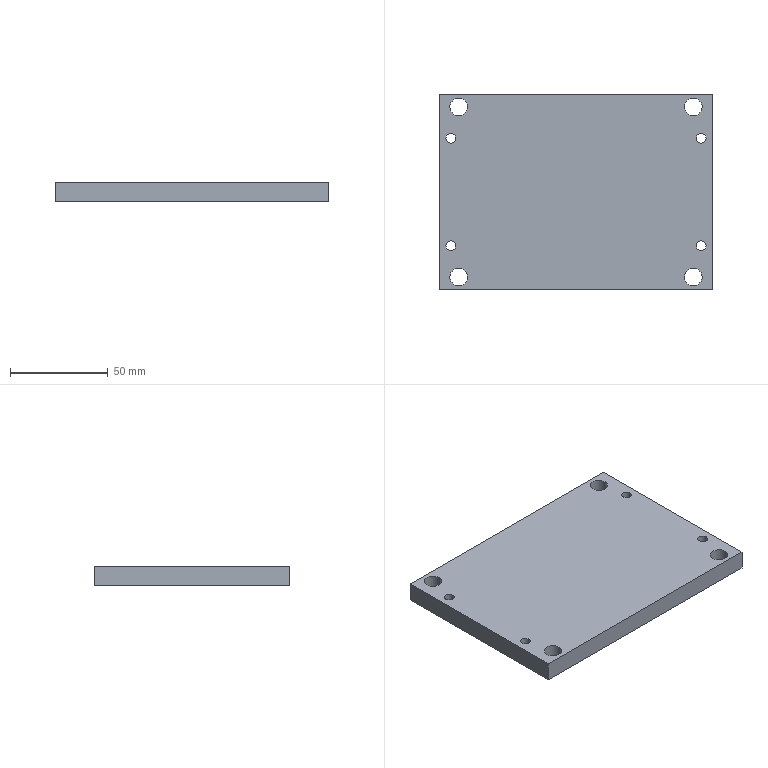Part | STEP file | B04 | 1 solid | 22 faces | box 140 x 100 x 10 mm | volume 136670 mm3 | cylinder 16 | plane 6 | commonest cylinder face diameters 5 x8 9 x8